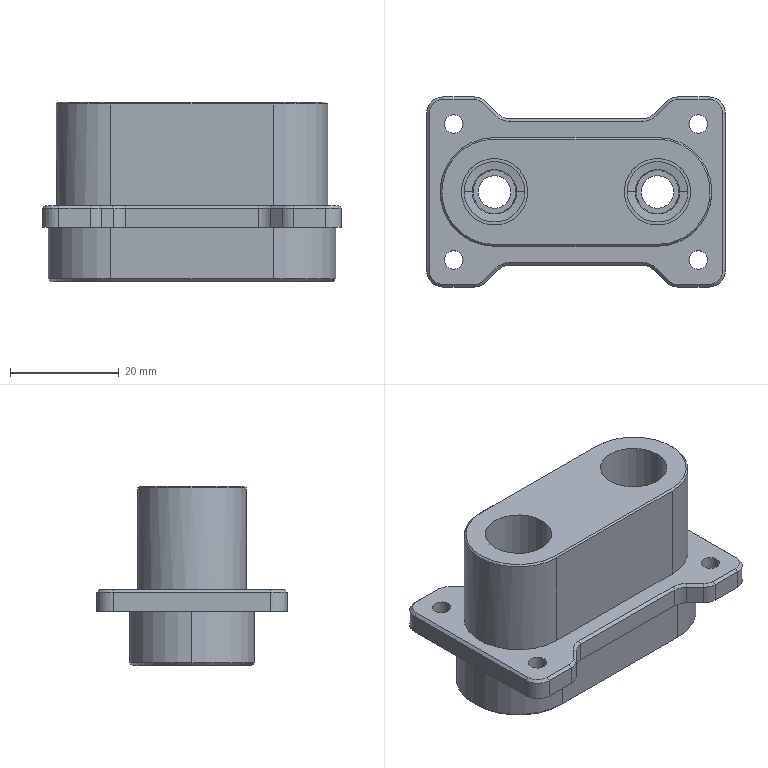NC program | NX | posted with a generic post | part box 55 x 35 x 33 mm
Lines 1800 to 2805 of 2805:
(PLANAR_MILL_3 , TOOL : D50面刀)
N3598 T01 M6
N3600 G54
N3602 G17 G0 G90 X-0.5 Y-54.499 S3500 M3
N3604 G43 Z30. H1
N3606 Z2.
N3608 G94 G1 Z0. F800.
N3610 Y-27.499
N3612 Y27.501
N3614 Y54.501
N3616 Z2.
N3618 G0 Z30.
N3620 M5
(DRILLING_2 , TOOL : D6点钻)
N3622 T03 M6
N3624 G54
N3626 G17 G0 G90 X0. Y15.001 S3000 M3
N3628 G43 Z30. H3
N3630 G94 G81 G98 Z-1.5 F200. R3.
N3632 Y-14.999
N3634 G80
N3636 G0 X0. Y-14.999 Z30.
N3638 M5
(DRILLING_2_COPY , TOOL : D6.5钻头)
N3640 T07 M6
N3642 G54
N3644 G17 G0 G90 X0. Y15.001 S3000 M3
N3646 G43 Z30. H7
N3648 G94 G83 G98 Z-22. F200. Q2. R3.
N3650 Y-14.999
N3652 G80
N3654 G0 X0. Y-14.999 Z30.
N3656 M5
(ADAPTIVE_MILLING_1 , TOOL : D4开粗)
N3658 T09 M6
N3660 G54
N3662 G17 G0 G90 X0. Y15.001 S4500 M3
N3664 G43 Z30. H9
N3666 Z-4.8
N3668 G94 G1 Z-7.8 F600.
N3670 X-0.129 Y14.749
N3672 X-0.242 Y14.488
N3674 G3 X-0.003 Y14.024 R0.405
N3676 X0.939 Y14.457 R0.821
N3678 X-0.266 Y13.936 R-1.092
N3680 X0.641 Y16.006 R1.139
N3682 X-0.135 Y13.792 R-1.2
N3684 X0.189 Y16.285 R-1.257
N3686 X-0.057 Y13.669 R-1.315
N3688 X-0.094 Y16.411 R-1.375
N3690 X0.246 Y13.558 R-1.437
N3692 X-0.727 Y16.35 R-1.502
N3694 X1.283 Y14.005 R-1.573
N3696 X-1.561 Y14.435 R-1.648
N3698 X0.93 Y16.529 R-1.728
N3700 X-0.224 Y13.182 R-1.807
N3702 X-0.149 Y16.926 R-1.885
N3704 X0.765 Y13.148 R-1.963
N3706 X-1.585 Y16.341 R-2.046
N3708 X2.2 Y14.888 R-2.133
N3710 X-1.676 Y13.511 R-2.223
N3712 X1.16 Y17.076 R-2.313
N3714 X-0.504 Y12.623 R-2.402
N3716 X-0.075 Y17.543 R-2.49
N3718 X0.822 Y12.509 R-2.58
N3720 X-1.537 Y17.235 R-2.671
N3722 X2.464 Y13.603 R-2.766
N3724 X-2.879 Y14.768 R-2.865
N3726 X2.637 Y16.518 R-2.965
N3728 X-1.875 Y12.542 R-3.065
N3730 X1.226 Y17.993 R-3.166
N3732 X-0.534 Y11.745 R-3.264
N3734 X0.001 Y18.424 R-3.364
N3736 X0.748 Y11.571 R-3.464
N3738 X-1.722 Y18.179 R-3.566
N3740 X2.827 Y12.556 R-3.671
N3742 X-3.497 Y16.517 R-3.778
N3744 X3.966 Y14.932 R-3.886
N3746 X-3.627 Y13.383 R-3.967
N3748 X-1.737 Y11.432 R4.253
N3750 X0.797 Y11.111 R4.23
N3752 X-0.275 Y18.963 R3.972
N3754 X-2.608 Y17.994 R4.267
N3756 X-3.635 Y16.6 R4.397
N3758 X-3.329 Y16.036 R0.404
N3760 G1 X-2.808 Y15.954
N3762 X-2.66 Y15.93 Z-7.796
N3764 X-2.512 Y15.906 Z-7.785
N3766 X-2.364 Y15.883 Z-7.766
N3768 X-2.216 Y15.859 Z-7.739
N3770 X-2.067 Y15.836 Z-7.705
N3772 X-1.919 Y15.812 Z-7.662
N3774 X-1.771 Y15.789 Z-7.61
N3776 X-1.623 Y15.765 Z-7.55
N3778 X-1.475 Y15.742 Z-7.479
N3780 X-1.327 Y15.718 Z-7.398
N3782 X-1.179 Y15.695 Z-7.305
N3784 X-1.03 Y15.671 Z-7.2
N3786 X-0.882 Y15.647 Z-7.08
N3788 X-0.734 Y15.624 Z-6.942
N3790 X-0.586 Y15.6 Z-6.784
N3792 X-0.438 Y15.577 Z-6.6
N3794 X-0.29 Y15.553 Z-6.38
N3796 X-0.142 Y15.53 Z-6.108
N3798 X0.007 Y15.506 Z-5.737
N3800 X0.155 Y15.483 Z-4.8
N3802 G0 Z30.
N3804 X0. Y-14.999
N3806 Z-4.8
N3808 G1 Z-7.8
N3810 X0.256 Y-15.118
N3812 X0.518 Y-15.221
N3814 G3 X0.976 Y-14.953 R0.405
N3816 X0.369 Y-13.975 R0.857
N3818 X1.084 Y-15.184 R-1.093
N3820 X-1.028 Y-14.397 R1.138
N3822 X1.202 Y-15.154 R-1.199
N3824 X0.162 Y-13.717 R1.254
N3826 X-1.274 Y-14.751 R1.254
N3828 X1.333 Y-14.977 R-1.313
N3830 X-1.405 Y-15.138 R-1.374
N3832 X1.434 Y-14.72 R-1.435
N3834 X-1.388 Y-15.647 R-1.5
N3836 X1.29 Y-14.036 R-1.568
N3838 X-0.646 Y-16.527 R-1.639
N3840 X-1.035 Y-13.545 R-1.718
N3842 X1.721 Y-15.592 R-1.799
N3844 X-1.921 Y-14.837 R-1.878
N3846 X1.97 Y-14.731 R-1.955
N3848 X-1.873 Y-15.89 R-2.035
N3850 X1.394 Y-13.329 R-2.119
N3852 X-0.326 Y-17.203 R-2.207
N3854 X-1.392 Y-13.08 R-2.298
N3856 X2.121 Y-16.152 R-2.39
N3858 X-2.482 Y-14.463 R-2.48
N3860 X2.6 Y-14.786 R-2.57
N3862 X-2.578 Y-15.829 R-2.662
N3864 X2.3 Y-13.389 R-2.754
N3866 X-1.599 Y-17.398 R-2.85
N3868 X0.052 Y-11.975 R-2.949
N3870 X1.394 Y-17.739 R-3.05
N3872 X-2.438 Y-12.886 R-3.152
N3874 X3.002 Y-16.331 R-3.253
N3876 X-3.334 Y-14.244 R-3.354
N3878 X3.496 Y-14.978 R-3.454
N3880 X-3.499 Y-15.895 R-3.557
N3882 X3.177 Y-13.068 R-3.661
N3884 X-2.495 Y-17.874 R-3.766
N3886 X1.602 Y-11.392 R-3.873
N3888 X-2.9 Y-17.696 R3.952
N3890 X1.112 Y-18.811 R4.004
N3892 X2.209 Y-18.299 R5.628
N3894 X3.509 Y-16.854 R4.555
N3896 X3.957 Y-15.368 R4.778
N3898 X-1.887 Y-11.514 R3.976
N3900 X-3.667 Y-13.476 R4.151
N3902 X-3.935 Y-14.461 R4.173
N3904 X-2.9 Y-17.696 R4.009
N3906 X-2.012 Y-18.42 R5.481
N3908 X-0.2 Y-18.967 R4.634
N3910 X0.198 Y-18.501 R0.404
N3912 G1 X0.117 Y-17.979
N3914 X0.094 Y-17.831 Z-7.796
N3916 X0.071 Y-17.683 Z-7.785
N3918 X0.048 Y-17.534 Z-7.766
N3920 X0.025 Y-17.386 Z-7.739
N3922 X0.002 Y-17.238 Z-7.705
N3924 X-0.021 Y-17.09 Z-7.662
N3926 X-0.044 Y-16.942 Z-7.61
N3928 X-0.067 Y-16.793 Z-7.55
N3930 X-0.09 Y-16.645 Z-7.479
N3932 X-0.113 Y-16.497 Z-7.398
N3934 X-0.136 Y-16.349 Z-7.305
N3936 X-0.159 Y-16.2 Z-7.2
N3938 X-0.182 Y-16.052 Z-7.08
N3940 X-0.205 Y-15.904 Z-6.942
N3942 X-0.228 Y-15.756 Z-6.784
N3944 X-0.251 Y-15.607 Z-6.6
N3946 X-0.274 Y-15.459 Z-6.38
N3948 X-0.297 Y-15.311 Z-6.108
N3950 X-0.32 Y-15.163 Z-5.737
N3952 X-0.343 Y-15.015 Z-4.8
N3954 G0 Z30.
N3956 X0.385 Y15.694
N3958 Z-14.808
N3960 G1 X0.366 Y15.659 Z-15.055
N3962 X0.346 Y15.624 Z-15.153
N3964 X0.327 Y15.59 Z-15.225
N3966 X0.308 Y15.555 Z-15.283
N3968 X0.289 Y15.521 Z-15.332
N3970 X0.269 Y15.486 Z-15.374
N3972 X0.25 Y15.451 Z-15.41
N3974 X0.231 Y15.417 Z-15.442
N3976 X0.212 Y15.382 Z-15.469
N3978 X0.192 Y15.347 Z-15.494
N3980 X0.173 Y15.313 Z-15.515
N3982 X0.154 Y15.278 Z-15.534
N3984 X0.135 Y15.244 Z-15.55
N3986 X0.115 Y15.209 Z-15.564
N3988 X0.096 Y15.174 Z-15.575
N3990 X0.077 Y15.14 Z-15.584
N3992 X0.058 Y15.105 Z-15.591
N3994 X0.038 Y15.07 Z-15.596
N3996 X0.019 Y15.036 Z-15.599
N3998 X0. Y15.001 Z-15.6
N4000 X-0.138 Y14.758
N4002 X-0.263 Y14.507
N4004 G3 X-0.003 Y14.009 R0.404
N4006 X1.035 Y14.662 R0.895
N4008 X-0.259 Y13.931 R-1.093
N4010 X0.69 Y15.972 R1.138
N4012 X-0.255 Y13.815 R-1.2
N4014 X0.323 Y16.258 R-1.256
N4016 X-0.104 Y13.671 R-1.314
N4018 X-0.01 Y16.413 R-1.375
N4020 X0.125 Y13.545 R-1.436
N4022 X-0.47 Y16.459 R-1.5
N4024 X0.816 Y13.613 R-1.568
N4026 X-1.524 Y15.656 R-1.64
N4028 X1.466 Y16.021 R-1.718
N4030 X0.776 Y13.371 R-1.792
N4032 X0.564 Y16.712 R1.809
N4034 X-1.709 Y14.424 R1.81
N4036 X-0.985 Y13.495 R1.84
N4038 X-0.425 Y13.703 R0.404
N4040 G1 X-0.213 Y14.227
N4042 X-0.184 Y14.3 Z-15.598
N4044 X-0.154 Y14.374 Z-15.592
N4046 X-0.124 Y14.447 Z-15.582
N4048 X-0.095 Y14.521 Z-15.568
N4050 X-0.065 Y14.594 Z-15.55
N4052 X-0.035 Y14.668 Z-15.527
N4054 X-0.005 Y14.741 Z-15.5
N4056 X0.024 Y14.814 Z-15.468
N4058 X0.054 Y14.888 Z-15.43
N4060 X0.084 Y14.961 Z-15.388
N4062 X0.113 Y15.035 Z-15.339
N4064 X0.143 Y15.108 Z-15.283
N4066 X0.173 Y15.182 Z-15.219
N4068 X0.203 Y15.255 Z-15.147
N4070 X0.232 Y15.329 Z-15.063
N4072 X0.262 Y15.402 Z-14.966
N4074 X0.292 Y15.476 Z-14.85
N4076 X0.321 Y15.549 Z-14.706
N4078 X0.351 Y15.623 Z-14.51
N4080 X0.381 Y15.696 Z-14.015
N4082 G0 Z30.
N4084 X-0.869 Y15.151
N4086 Z-13.743
N4088 G1 X-0.826 Y15.144 Z-14.018
N4090 X-0.783 Y15.136 Z-14.127
N4092 X-0.739 Y15.129 Z-14.207
N4094 X-0.696 Y15.121 Z-14.272
N4096 X-0.652 Y15.114 Z-14.326
N4098 X-0.609 Y15.106 Z-14.373
N4100 X-0.565 Y15.099 Z-14.413
N4102 X-0.522 Y15.091 Z-14.449
N4104 X-0.478 Y15.084 Z-14.48
N4106 X-0.435 Y15.076 Z-14.507
N4108 X-0.391 Y15.069 Z-14.531
N4110 X-0.348 Y15.061 Z-14.551
N4112 X-0.304 Y15.054 Z-14.569
N4114 X-0.261 Y15.046 Z-14.584
N4116 X-0.217 Y15.039 Z-14.597
N4118 X-0.174 Y15.031 Z-14.607
N4120 X-0.13 Y15.024 Z-14.615
N4122 X-0.087 Y15.016 Z-14.621
N4124 X-0.043 Y15.009 Z-14.624
N4126 X0. Y15.001 Z-14.625
N4128 X1.341 Y14.769
N4130 G3 X1.768 Y14.981 R0.405
N4132 X1.68 Y15.869 R1.058
N4134 X-0.699 Y13.247 R-1.887
N4136 X1.87 Y15.278 R1.895
N4138 X1.36 Y16.321 R2.098
N4140 X0.834 Y16.355 R0.441
N4142 G1 X0.203 Y15.881 Z-14.525
N4144 X-0.884 Y15.061 F6000.
N4146 X-1.514 Y14.586 Z-14.625 F600.
N4148 G3 X-1.567 Y13.946 R0.445
N4150 X0.006 Y13.107 R1.979
N4152 G1 X0.614 Y13.212
N4154 G3 X0.935 Y13.651 R0.441
N4156 X0.713 Y14.025 Z-14.568 R0.479
N4158 G1 X0.45 Y14.237 Z-14.525
N4160 X-0.83 Y15.27 F6000.
N4162 X-1.222 Y15.579 Z-14.588 F600.
N4164 G3 X-1.502 Y15.632 Z-14.625 R0.464
N4166 X-1.871 Y15.269 R0.436
N4168 X-1.41 Y14.811 R0.404
N4170 G1 X-0.879 Y14.892
N4172 X-0.792 Y14.906 Z-14.623
N4174 X-0.704 Y14.919 Z-14.616
N4176 X-0.617 Y14.932 Z-14.605
N4178 X-0.53 Y14.946 Z-14.589
N4180 X-0.443 Y14.959 Z-14.569
N4182 X-0.355 Y14.973 Z-14.544
N4184 X-0.268 Y14.986 Z-14.513
N4186 X-0.181 Y14.999 Z-14.478
N4188 X-0.094 Y15.013 Z-14.436
N4190 X-0.007 Y15.026 Z-14.389
N4192 X0.081 Y15.04 Z-14.334
N4194 X0.168 Y15.053 Z-14.272
N4196 X0.255 Y15.066 Z-14.201
N4198 X0.342 Y15.08 Z-14.12
N4200 X0.43 Y15.093 Z-14.027
N4202 X0.517 Y15.107 Z-13.919
N4204 X0.604 Y15.12 Z-13.79
N4206 X0.691 Y15.133 Z-13.629
N4208 X0.779 Y15.147 Z-13.411
N4210 X0.866 Y15.16 Z-12.86
N4212 G0 Z30.
N4214 X-1.778 Y15.285
N4216 Z-10.875
N4218 G1 X-1.689 Y15.271 Z-11.437
N4220 X-1.6 Y15.257 Z-11.659
N4222 X-1.511 Y15.243 Z-11.823
N4224 X-1.422 Y15.228 Z-11.955
N4226 X-1.333 Y15.214 Z-12.065
N4228 X-1.245 Y15.2 Z-12.16
N4230 X-1.156 Y15.186 Z-12.243
N4232 X-1.067 Y15.172 Z-12.315
N4234 X-0.978 Y15.157 Z-12.378
N4236 X-0.889 Y15.143 Z-12.434
N4238 X-0.8 Y15.129 Z-12.482
N4240 X-0.711 Y15.115 Z-12.525
N4242 X-0.622 Y15.101 Z-12.561
N4244 X-0.533 Y15.086 Z-12.592
N4246 X-0.444 Y15.072 Z-12.618
N4248 X-0.356 Y15.058 Z-12.639
N4250 X-0.267 Y15.044 Z-12.655
N4252 X-0.178 Y15.03 Z-12.666
N4254 X-0.089 Y15.015 Z-12.673
N4256 X0. Y15.001 Z-12.675
N4258 X1.43 Y14.773
N4260 G3 X1.866 Y15.015 R0.405
N4262 X1.486 Y16.355 R1.415
N4264 X1.905 Y14.323 R-2.024
N4266 X-0.837 Y17.008 R2.063
N4268 X2.088 Y14.359 R-2.177
N4270 X-1.256 Y16.961 R2.23
N4272 X2.206 Y14.21 R-2.332
N4274 X-1.552 Y16.948 R2.399
N4276 X2.348 Y14.118 R-2.495
N4278 X-1.87 Y16.885 R2.569
N4280 X2.474 Y13.982 R-2.662
N4282 X-1.263 Y17.505 R2.721
N4284 X0.195 Y17.796 R-2.802
N4286 X1.713 Y12.773 R-2.804
N4288 G1 X2.27 Y13.347
N4290 G3 X2.079 Y13.968 R0.404
N4292 G1 X1.576 Y14.144
N4294 X1.434 Y14.194 Z-12.671
N4296 X1.293 Y14.244 Z-12.66
N4298 X1.151 Y14.294 Z-12.641
N4300 X1.01 Y14.344 Z-12.614
N4302 X0.868 Y14.393 Z-12.58
N4304 X0.727 Y14.443 Z-12.537
N4306 X0.585 Y14.493 Z-12.485
N4308 X0.444 Y14.543 Z-12.425
N4310 X0.302 Y14.593 Z-12.354
N4312 X0.161 Y14.642 Z-12.273
N4314 X0.019 Y14.692 Z-12.18
N4316 X-0.122 Y14.742 Z-12.075
N4318 X-0.264 Y14.792 Z-11.955
N4320 X-0.405 Y14.842 Z-11.817
N4322 X-0.547 Y14.891 Z-11.659
N4324 X-0.688 Y14.941 Z-11.475
N4326 X-0.83 Y14.991 Z-11.255
N4328 X-0.971 Y15.041 Z-10.983
N4330 X-1.113 Y15.091 Z-10.612
N4332 X-1.254 Y15.14 Z-9.675
N4334 G0 Z30.
N4336 X2.371 Y15.456
N4338 Z-9.002
N4340 G1 X2.236 Y15.45 Z-9.844
N4342 X2.101 Y15.444 Z-10.178
N4344 X1.966 Y15.437 Z-10.423
N4346 X1.832 Y15.431 Z-10.621
N4348 X1.697 Y15.425 Z-10.787
N4350 X1.562 Y15.419 Z-10.929
N4352 X1.427 Y15.412 Z-11.052
N4354 X1.292 Y15.406 Z-11.16
N4356 X1.158 Y15.4 Z-11.255
N4358 X1.023 Y15.394 Z-11.339
N4360 X0.888 Y15.388 Z-11.411
N4362 X0.753 Y15.381 Z-11.475
N4364 X0.619 Y15.375 Z-11.529
N4366 X0.484 Y15.369 Z-11.576
N4368 X0.349 Y15.363 Z-11.614
N4370 X0.214 Y15.356 Z-11.645
N4372 X0.08 Y15.35 Z-11.669
N4374 X-0.055 Y15.344 Z-11.686
N4376 X-0.19 Y15.338 Z-11.697
N4378 X-0.325 Y15.332 Z-11.7
N4380 X-2.421 Y15.235
N4382 G3 X-2.769 Y15. R0.406
N4384 X-2.632 Y13.669 R1.657
N4386 X1.495 Y17.577 R-2.968
N4388 X-2.973 Y15.349 R3.011
N4390 X-0.449 Y11.883 R2.924
N4392 X-3.058 Y15.817 R-3.154
N4394 X0.563 Y11.714 R3.179
N4396 X-3.144 Y16.152 R-3.339
N4398 X-3.208 Y13.82 R3.199
N4400 X-0.797 Y11.676 R3.526
N4402 X2.393 Y12.559 R3.525
N4404 X3.134 Y16.368 R3.487
N4406 X-0.064 Y18.42 R3.491
N4408 X-3.169 Y16.284 R3.482
N4410 X-3.401 Y14.651 R3.82
N4412 X-2.864 Y14.325 R0.404
N4414 G1 X-2.355 Y14.508
N4416 X-2.214 Y14.558 Z-11.696
N4418 X-2.073 Y14.609 Z-11.685
N4420 X-1.932 Y14.66 Z-11.666
N4422 X-1.791 Y14.71 Z-11.639
N4424 X-1.649 Y14.761 Z-11.605
N4426 X-1.508 Y14.811 Z-11.562
N4428 X-1.367 Y14.862 Z-11.51
N4430 X-1.226 Y14.913 Z-11.45
N4432 X-1.085 Y14.963 Z-11.379
N4434 X-0.943 Y15.014 Z-11.298
N4436 X-0.802 Y15.065 Z-11.205
N4438 X-0.661 Y15.115 Z-11.1
N4440 X-0.52 Y15.166 Z-10.98
N4442 X-0.379 Y15.217 Z-10.842
N4444 X-0.238 Y15.267 Z-10.684
N4446 X-0.096 Y15.318 Z-10.5
N4448 X0.045 Y15.368 Z-10.28
N4450 X0.186 Y15.419 Z-10.008
N4452 X0.327 Y15.47 Z-9.637
N4454 X0.468 Y15.52 Z-8.7
N4456 G0 Z30.
N4458 X-2.288 Y16.542
N4460 Z-6.75
N4462 G1 X-2.228 Y16.405 Z-7.687
N4464 X-2.169 Y16.267 Z-8.058
N4466 X-2.109 Y16.129 Z-8.33
N4468 X-2.05 Y15.992 Z-8.55
N4470 X-1.991 Y15.854 Z-8.734
N4472 X-1.931 Y15.716 Z-8.892
N4474 X-1.872 Y15.578 Z-9.03
N4476 X-1.812 Y15.441 Z-9.15
N4478 X-1.753 Y15.303 Z-9.255
N4480 X-1.693 Y15.165 Z-9.348
N4482 X-1.634 Y15.027 Z-9.429
N4484 X-1.574 Y14.89 Z-9.5
N4486 X-1.515 Y14.752 Z-9.56
N4488 X-1.456 Y14.614 Z-9.612
N4490 X-1.396 Y14.477 Z-9.655
N4492 X-1.337 Y14.339 Z-9.689
N4494 X-1.277 Y14.201 Z-9.716
N4496 X-1.218 Y14.063 Z-9.735
N4498 X-1.158 Y13.926 Z-9.746
N4500 X-1.099 Y13.788 Z-9.75
N4502 X-0.244 Y11.808
N4504 G3 X-0.007 Y11.587 R0.41
N4506 X1.746 Y11.87 R2.296
N4508 X-1.475 Y11.723 R-3.595
N4510 X1.012 Y11.402 R4.173
N4512 X2.401 Y17.934 R3.738
N4514 X-0.902 Y11.303 R-3.794
N4516 X3.34 Y12.865 R3.696
N4518 X2.906 Y12.305 R-3.963
N4520 X3.947 Y14.576 R4.
N4522 X3.863 Y15.929 R3.929
N4524 X-3.627 Y13.383 R-3.971
N4526 X-1.737 Y11.432 R4.253
N4528 G1 X-1.702 Y11.419
N4530 G3 X-1.173 Y11.694 R0.404
N4532 G1 X-1.03 Y12.23
N4534 X-0.991 Y12.375 Z-9.746
N4536 X-0.952 Y12.519 Z-9.735
N4538 X-0.913 Y12.664 Z-9.716
N4540 X-0.875 Y12.809 Z-9.689
N4542 X-0.836 Y12.954 Z-9.655
N4544 X-0.797 Y13.099 Z-9.612
N4546 X-0.758 Y13.244 Z-9.56
N4548 X-0.719 Y13.389 Z-9.5
N4550 X-0.681 Y13.534 Z-9.429
N4552 X-0.642 Y13.679 Z-9.348
N4554 X-0.603 Y13.824 Z-9.255
N4556 X-0.564 Y13.968 Z-9.15
N4558 X-0.525 Y14.113 Z-9.03
N4560 X-0.487 Y14.258 Z-8.892
N4562 X-0.448 Y14.403 Z-8.734
N4564 X-0.409 Y14.548 Z-8.55
N4566 X-0.37 Y14.693 Z-8.33
N4568 X-0.331 Y14.838 Z-8.058
N4570 X-0.293 Y14.983 Z-7.687
N4572 X-0.254 Y15.128 Z-6.75
N4574 G0 Z30.
N4576 X-0.707 Y-14.623
N4578 Z-14.799
N4580 G1 X-0.672 Y-14.641 Z-15.049
N4582 X-0.637 Y-14.66 Z-15.148
N4584 X-0.601 Y-14.679 Z-15.221
N4586 X-0.566 Y-14.698 Z-15.28
N4588 X-0.53 Y-14.717 Z-15.329
N4590 X-0.495 Y-14.736 Z-15.371
N4592 X-0.46 Y-14.754 Z-15.408
N4594 X-0.424 Y-14.773 Z-15.44
N4596 X-0.389 Y-14.792 Z-15.468
N4598 X-0.354 Y-14.811 Z-15.493
N4600 X-0.318 Y-14.83 Z-15.514
N4602 X-0.283 Y-14.848 Z-15.533
N4604 X-0.248 Y-14.867 Z-15.549
N4606 X-0.212 Y-14.886 Z-15.563
N4608 X-0.177 Y-14.905 Z-15.575
N4610 X-0.141 Y-14.924 Z-15.584
N4612 X-0.106 Y-14.942 Z-15.591
N4614 X-0.071 Y-14.961 Z-15.596
N4616 X-0.035 Y-14.98 Z-15.599
N4618 X0. Y-14.999 Z-15.6
N4620 X0.246 Y-15.133
N4622 X0.5 Y-15.254
N4624 G3 X0.989 Y-15.001 R0.404
N4626 X0.969 Y-14.558 R0.61
N4628 X-0.684 Y-14.148 R1.058
N4630 X1.037 Y-15.351 R-1.093
N4632 X-0.032 Y-13.81 R1.113
N4634 X1.028 Y-15.609 R-1.192
N4636 X-0.369 Y-13.757 R1.234
N4638 X0.991 Y-15.844 R-1.298
N4640 X-0.537 Y-13.698 R1.35
N4642 X0.987 Y-16.015 R-1.412
N4644 X-0.639 Y-13.612 R1.468
N4646 X0.952 Y-16.205 R-1.531
N4648 X-0.598 Y-13.46 R1.592
N4650 X0.848 Y-16.429 R-1.657
N4652 X-0.562 Y-13.309 R1.721
N4654 X0.661 Y-16.667 R-1.788
N4656 X1.295 Y-16.249 R2.062
N4658 X1.558 Y-14.082 R1.848
N4660 X-0.535 Y-13.271 R1.868
N4662 X-1.694 Y-14.366 R1.939
N4664 X-1.587 Y-15.83 R1.783
N4666 X-1.31 Y-16.22 R0.989
N4668 G1 X-1.249 Y-16.282
N4670 G3 X-0.889 Y-16.554 R0.935
N4672 G1 X-0.769 Y-16.617
N4674 G3 X-0.314 Y-16.761 R0.988
N4676 X1.522 Y-15.95 R1.752
N4678 G1 X1.616 Y-15.802
N4680 G3 X1.349 Y-15.255 R0.404
N4682 G1 X0.797 Y-15.107
N4684 X0.72 Y-15.086 Z-15.598
N4686 X0.643 Y-15.065 Z-15.592
N4688 X0.566 Y-15.044 Z-15.582
N4690 X0.489 Y-15.023 Z-15.568
N4692 X0.412 Y-15.002 Z-15.549
N4694 X0.335 Y-14.982 Z-15.526
N4696 X0.258 Y-14.961 Z-15.499
N4698 X0.18 Y-14.94 Z-15.467
N4700 X0.103 Y-14.919 Z-15.429
N4702 X0.026 Y-14.898 Z-15.386
N4704 X-0.051 Y-14.877 Z-15.337
N4706 X-0.128 Y-14.857 Z-15.281
N4708 X-0.205 Y-14.836 Z-15.217
N4710 X-0.282 Y-14.815 Z-15.143
N4712 X-0.359 Y-14.794 Z-15.059
N4714 X-0.436 Y-14.773 Z-14.961
N4716 X-0.514 Y-14.753 Z-14.844
N4718 X-0.591 Y-14.732 Z-14.699
N4720 X-0.668 Y-14.711 Z-14.501
N4722 X-0.745 Y-14.69 Z-14.003
N4724 G0 Z30.
N4726 X-0.862 Y-14.82
N4728 Z-13.745
N4730 G1 X-0.819 Y-14.829 Z-14.02
N4732 X-0.775 Y-14.838 Z-14.129
N4734 X-0.732 Y-14.847 Z-14.209
N4736 X-0.689 Y-14.856 Z-14.273
N4738 X-0.646 Y-14.865 Z-14.327
N4740 X-0.603 Y-14.874 Z-14.373
N4742 X-0.56 Y-14.883 Z-14.414
N4744 X-0.517 Y-14.892 Z-14.449
N4746 X-0.474 Y-14.901 Z-14.48
N4748 X-0.431 Y-14.91 Z-14.507
N4750 X-0.388 Y-14.918 Z-14.531
N4752 X-0.345 Y-14.927 Z-14.552
N4754 X-0.302 Y-14.936 Z-14.569
N4756 X-0.258 Y-14.945 Z-14.584
N4758 X-0.215 Y-14.954 Z-14.597
N4760 X-0.172 Y-14.963 Z-14.607
N4762 X-0.129 Y-14.972 Z-14.615
N4764 X-0.086 Y-14.981 Z-14.621
N4766 X-0.043 Y-14.99 Z-14.624
N4768 X0. Y-14.999 Z-14.625
N4770 X1.33 Y-15.274
N4772 G3 X1.79 Y-15.02 R0.405
N4774 X1.668 Y-14.109 R1.205
N4776 X-1.122 Y-16.519 R-1.888
N4778 X1.867 Y-14.703 R1.896
N4780 G1 X1.825 Y-14.559
N4782 G3 X1.503 Y-14.277 R0.402
N4784 X1.148 Y-14.39 Z-14.576 R0.448
N4786 G1 X0.818 Y-14.625 Z-14.525
N4788 X0.311 Y-14.981 F6000.
N4790 X0.212 Y-15.011
N4792 X0.109 Y-15.019
N4794 X-0.054 Y-15.006
N4796 X-0.217 Y-15.007
N4798 X-0.861 Y-15.195
N4800 X-1.455 Y-15.376 Z-14.604 F600.
N4802 X-1.525 Y-15.421 Z-14.614
N4804 X-1.589 Y-15.475 Z-14.625
N4806 G3 X-1.659 Y-15.89 R0.402
N4808 X0.332 Y-16.844 R1.847
N4810 X1.409 Y-16.235 R1.717
N4812 G1 X1.601 Y-16.008
N4814 G3 X1.368 Y-15.382 R0.404
N4816 G1 X0.848 Y-15.254
N4818 X0.762 Y-15.232 Z-14.623
N4820 X0.677 Y-15.211 Z-14.616
N4822 X0.591 Y-15.19 Z-14.605
N4824 X0.505 Y-15.169 Z-14.589
N4826 X0.42 Y-15.148 Z-14.569
N4828 X0.334 Y-15.126 Z-14.544
N4830 X0.249 Y-15.105 Z-14.513
N4832 X0.163 Y-15.084 Z-14.478
N4834 X0.077 Y-15.063 Z-14.436
N4836 X-0.008 Y-15.042 Z-14.389
N4838 X-0.094 Y-15.021 Z-14.334
N4840 X-0.179 Y-14.999 Z-14.272
N4842 X-0.265 Y-14.978 Z-14.202
N4844 X-0.351 Y-14.957 Z-14.121
N4846 X-0.436 Y-14.936 Z-14.028
N4848 X-0.522 Y-14.915 Z-13.92
N4850 X-0.607 Y-14.893 Z-13.79
N4852 X-0.693 Y-14.872 Z-13.63
N4854 X-0.779 Y-14.851 Z-13.412
N4856 X-0.864 Y-14.83 Z-12.861
N4858 G0 Z30.
N4860 X-0.27 Y-16.774
N4862 Z-10.88
N4864 G1 X-0.256 Y-16.685 Z-11.44
N4866 X-0.243 Y-16.596 Z-11.662
N4868 X-0.229 Y-16.508 Z-11.825
N4870 X-0.216 Y-16.419 Z-11.957
N4872 X-0.202 Y-16.33 Z-12.067
N4874 X-0.189 Y-16.241 Z-12.162
N4876 X-0.175 Y-16.153 Z-12.244
N4878 X-0.162 Y-16.064 Z-12.316
N4880 X-0.148 Y-15.975 Z-12.379
N4882 X-0.135 Y-15.886 Z-12.434
N4884 X-0.121 Y-15.798 Z-12.483
N4886 X-0.108 Y-15.709 Z-12.525
N4888 X-0.094 Y-15.62 Z-12.561
N4890 X-0.081 Y-15.531 Z-12.592
N4892 X-0.067 Y-15.443 Z-12.618
N4894 X-0.054 Y-15.354 Z-12.639
N4896 X-0.04 Y-15.265 Z-12.655
N4898 X-0.027 Y-15.176 Z-12.666
N4900 X-0.013 Y-15.088 Z-12.673
N4902 X0. Y-14.999 Z-12.675
N4904 X0.217 Y-13.568
N4906 G3 X-0.013 Y-13.141 R0.405
N4908 X-1.218 Y-13.398 R1.301
N4910 X0.937 Y-13.202 R-2.024
N4912 X-1.342 Y-13.316 R2.146
N4914 X2.011 Y-14.172 R-2.17
N4916 X-1.686 Y-13.424 R2.281
N4918 X1.713 Y-13.421 R-2.325
N4920 X-1.811 Y-16.706 R-2.409
N4922 X0.815 Y-12.621 R-2.497
N4924 X-1.873 Y-16.879 R2.571
N4926 X0.993 Y-12.51 R-2.663
N4928 X-2.552 Y-16.146 R2.716
N4930 X1.15 Y-17.551 R2.8
N4932 X-2.552 Y-16.146 R-2.8
N4934 X1.625 Y-12.713 R-2.802
N4936 G1 X1.555 Y-12.659
N4938 G3 X0.951 Y-12.873 R0.404
N4940 G1 X0.785 Y-13.385
N4942 X0.738 Y-13.528 Z-12.671
N4944 X0.692 Y-13.67 Z-12.66
N4946 X0.646 Y-13.813 Z-12.641
N4948 X0.599 Y-13.956 Z-12.614
N4950 X0.553 Y-14.098 Z-12.58
N4952 X0.507 Y-14.241 Z-12.537
N4954 X0.46 Y-14.384 Z-12.485
N4956 X0.414 Y-14.526 Z-12.425
N4958 X0.368 Y-14.669 Z-12.354
N4960 X0.321 Y-14.812 Z-12.273
N4962 X0.275 Y-14.954 Z-12.18
N4964 X0.229 Y-15.097 Z-12.075
N4966 X0.182 Y-15.24 Z-11.955
N4968 X0.136 Y-15.382 Z-11.817
N4970 X0.09 Y-15.525 Z-11.659
N4972 X0.043 Y-15.668 Z-11.475
N4974 X-0.003 Y-15.81 Z-11.255
N4976 X-0.049 Y-15.953 Z-10.983
N4978 X-0.096 Y-16.096 Z-10.612
N4980 X-0.142 Y-16.238 Z-9.675
N4982 G0 Z30.
N4984 X2.41 Y-14.982
N4986 Z-8.954
N4988 G1 X2.273 Y-14.983 Z-9.811
N4990 X2.135 Z-10.151
N4992 X1.998 Y-14.984 Z-10.4
N4994 X1.861 Y-14.985 Z-10.601
N4996 X1.723 Y-14.986 Z-10.77
N4998 X1.586 Y-14.987 Z-10.915
N5000 X1.449 Y-14.988 Z-11.041
N5002 X1.311 Y-14.989 Z-11.151
N5004 X1.174 Y-14.99 Z-11.247
N5006 X1.037 Z-11.332
N5008 X0.9 Y-14.991 Z-11.406
N5010 X0.762 Y-14.992 Z-11.471
N5012 X0.625 Y-14.993 Z-11.526
N5014 X0.488 Y-14.994 Z-11.574
N5016 X0.35 Y-14.995 Z-11.613
N5018 X0.213 Y-14.996 Z-11.645
N5020 X0.076 Y-14.997 Z-11.669
N5022 X-0.062 Z-11.686
N5024 X-0.199 Y-14.998 Z-11.697
N5026 X-0.336 Y-14.999 Z-11.7
N5028 X-2.389 Y-15.012
N5030 G3 X-2.781 Y-15.33 R0.405
N5032 X-2.234 Y-16.943 R2.018
N5034 X-2.94 Y-14.56 R-2.973
N5036 X0.114 Y-18.147 R2.948
N5038 X-3.124 Y-14.486 R-3.154
N5040 X0.833 Y-18.227 R3.177
N5042 X-3.254 Y-14.201 R-3.338
N5044 X-3.208 Y-16.18 R3.137
N5046 X-0.797 Y-18.324 R3.526
N5048 X2.425 Y-17.408 R3.52
N5050 X3.418 Y-15.068 R3.616
N5052 X2.521 Y-12.69 R3.616
N5054 X0.617 Y-11.634 R3.679
N5056 X-3.375 Y-15.474 R3.425
N5058 X-2.955 Y-15.791 R0.405
N5060 G1 X-2.303 Y-15.749
N5062 X-2.154 Y-15.74 Z-11.696
N5064 X-2.004 Y-15.73 Z-11.685
N5066 X-1.854 Y-15.721 Z-11.666
N5068 X-1.705 Y-15.711 Z-11.639
N5070 X-1.555 Y-15.702 Z-11.605
N5072 X-1.405 Y-15.692 Z-11.562
N5074 X-1.255 Y-15.682 Z-11.51
N5076 X-1.106 Y-15.673 Z-11.45
N5078 X-0.956 Y-15.663 Z-11.379
N5080 X-0.806 Y-15.654 Z-11.298
N5082 X-0.657 Y-15.644 Z-11.205
N5084 X-0.507 Y-15.634 Z-11.1
N5086 X-0.357 Y-15.625 Z-10.98
N5088 X-0.208 Y-15.615 Z-10.842
N5090 X-0.058 Y-15.606 Z-10.684
N5092 X0.092 Y-15.596 Z-10.5
N5094 X0.241 Y-15.587 Z-10.28
N5096 X0.391 Y-15.577 Z-10.008
N5098 X0.541 Y-15.567 Z-9.637
N5100 X0.691 Y-15.558 Z-8.7
N5102 G0 Z30.
N5104 X-2.069 Y-13.396
N5106 Z-6.75
N5108 G1 X-2.017 Y-13.536 Z-7.687
N5110 X-1.965 Y-13.677 Z-8.058
N5112 X-1.913 Y-13.818 Z-8.33
N5114 X-1.861 Y-13.958 Z-8.55
N5116 X-1.809 Y-14.099 Z-8.734
N5118 X-1.757 Y-14.24 Z-8.892
N5120 X-1.705 Y-14.38 Z-9.03
N5122 X-1.653 Y-14.521 Z-9.15
N5124 X-1.601 Y-14.662 Z-9.255
N5126 X-1.549 Y-14.802 Z-9.348
N5128 X-1.496 Y-14.943 Z-9.429
N5130 X-1.444 Y-15.084 Z-9.5
N5132 X-1.392 Y-15.224 Z-9.56
N5134 X-1.34 Y-15.365 Z-9.612
N5136 X-1.288 Y-15.506 Z-9.655
N5138 X-1.236 Y-15.646 Z-9.689
N5140 X-1.184 Y-15.787 Z-9.716
N5142 X-1.132 Y-15.928 Z-9.735
N5144 X-1.08 Y-16.068 Z-9.746
N5146 X-1.028 Y-16.209 Z-9.75
N5148 X-0.312 Y-18.145
N5150 G3 X0.066 Y-18.409 R0.405
N5152 X2.195 Y-17.835 R2.605
N5154 X-0.666 Y-18.534 R-3.595
N5156 X3.626 Y-16.089 R3.498
N5158 X-0.834 Y-18.708 R-3.788
N5160 X3.412 Y-17.003 R3.692
N5162 X-3.579 Y-13.304 R-3.959
N5164 X-2.1 Y-18.356 R3.96
N5166 X3.776 Y-16.178 R3.955
N5168 X3.756 Y-13.743 R3.735
N5170 X-2.923 Y-17.666 R-3.959
N5172 X-1.194 Y-18.784 R4.225
N5174 X-0.67 Y-18.42 R0.404
N5176 G1 X-0.641 Y-17.882
N5178 X-0.633 Y-17.733 Z-9.746
N5180 X-0.625 Y-17.583 Z-9.735
N5182 X-0.617 Y-17.433 Z-9.716
N5184 X-0.609 Y-17.283 Z-9.689
N5186 X-0.601 Y-17.134 Z-9.655
N5188 X-0.593 Y-16.984 Z-9.612
N5190 X-0.585 Y-16.834 Z-9.56
N5192 X-0.577 Y-16.684 Z-9.5
N5194 X-0.569 Y-16.534 Z-9.429
N5196 X-0.561 Y-16.385 Z-9.348
N5198 X-0.553 Y-16.235 Z-9.255
N5200 X-0.545 Y-16.085 Z-9.15
N5202 X-0.536 Y-15.935 Z-9.03
N5204 X-0.528 Y-15.785 Z-8.892
N5206 X-0.52 Y-15.636 Z-8.734
N5208 X-0.512 Y-15.486 Z-8.55
N5210 X-0.504 Y-15.336 Z-8.33
N5212 X-0.496 Y-15.186 Z-8.058
N5214 X-0.488 Y-15.037 Z-7.687
N5216 X-0.48 Y-14.887 Z-6.75
N5218 G0 Z30.
N5220 M5
(DRILLING_2_COPY_COPY , TOOL : D7.9成型刀)
N5222 T10 M6
N5224 G54
N5226 G17 G0 G90 X0. Y15.001 S4000 M3
N5228 G43 Z30. H10
N5230 G94 G81 G98 Z-15.75 F80. R3.
N5232 Y-14.999
N5234 G80
N5236 G0 X0. Y-14.999 Z30.
N5238 M5
(PLANAR_MILL_5 , TOOL : D6点钻)
N5240 T03 M6
N5242 G54
N5244 G17 G0 G90 X-13.2 Y13.001 S3500 M3
N5246 G43 Z30. H3
N5248 Z0.5
N5250 G94 G1 Z-1.5 F800.
N5252 G3 X-11.2 Y15.001 R2.
N5254 G2 X0. Y26.201 R11.2
N5256 X11.2 Y15.001 R11.2
N5258 G1 Y-14.999
N5260 G2 X0. Y-26.199 R11.2
N5262 X-11.2 Y-14.999 R11.2
N5264 G1 Y15.001
N5266 G3 X-13.2 Y17.001 R2.
N5268 G1 Z0.5
N5270 G0 Z30.
(PLANAR_MILL_5_COPY , TOOL : D6点钻)
N5272 X-21. Y16.744
N5274 Z-19.
N5276 G1 Z-21.
N5278 G3 X-19. Y18.744 R2.
N5280 G1 Y24.501
N5282 G2 X-14.5 Y29.001 R4.5
N5284 G1 X14.5
N5286 G2 X19. Y24.501 R4.5
N5288 G1 Y18.744
N5290 G2 X17.682 Y15.562 R4.5
N5292 G1 X15.439 Y13.319
N5294 G3 X15. Y12.259 R1.5
N5296 G1 Y-12.256
N5298 G3 X15.439 Y-13.317 R1.5
N5300 G1 X17.682 Y-15.559
N5302 G2 X19. Y-18.741 R4.5
N5304 G1 Y-24.499
N5306 G2 X14.5 Y-28.999 R4.5
N5308 G1 X-14.5
N5310 G2 X-19. Y-24.499 R4.5
N5312 G1 Y-18.741
N5314 G2 X-17.682 Y-15.559 R4.5
N5316 G1 X-15.439 Y-13.317
N5318 G3 X-15. Y-12.256 R1.5
N5320 G1 Y12.259
N5322 G3 X-15.439 Y13.319 R1.5
N5324 G1 X-17.682 Y15.562
N5326 G2 X-19. Y18.744 R4.5
N5328 G3 X-21. Y20.744 R2.
N5330 G1 Z-19.
N5332 G0 Z30.
(DRILLING_3 , TOOL : D6点钻)
N5334 X-12.5 Y22.501 S3000
N5336 G81 G98 Z-20.7 F200. R-16.
N5338 Y-22.499
N5340 X12.5
N5342 Y22.501
N5344 G80
N5346 G0 X12.5 Y22.501 Z30.
N5348 M5
(PLANAR_MILL_7 , TOOL : D6精光)
N5350 T06 M6
N5352 G54
N5354 G17 G0 G90 X-19.2 Y13.001 S5500 M3
N5356 G43 Z30. H6
N5358 Z-17.
N5360 G94 G1 Z-19. F800.
N5362 G3 X-17.2 Y15.001 R2.
N5364 G2 X0. Y32.201 R17.2
N5366 X17.2 Y15.001 R17.2
N5368 G1 Y-14.999
N5370 G2 X0. Y-32.199 R17.2
N5372 X-17.2 Y-14.999 R17.2
N5374 G1 Y15.001
N5376 G3 X-19.2 Y17.001 R2.
N5378 G1 X-15. Y13.001
N5380 G3 X-13. Y15.001 R2.
N5382 G2 X0. Y28.001 R13.
N5384 X13. Y15.001 R13.
N5386 G1 Y-14.999
N5388 G2 X0. Y-27.999 R13.
N5390 X-13. Y-14.999 R13.
N5392 G1 Y15.001
N5394 G3 X-15. Y17.001 R2.
N5396 G1 X-19.032 Y17.539
N5398 Z-17.
N5400 G0 Z30.
(PLANAR_MILL_7_COPY , TOOL : D6精光)
N5402 X-17.197 Y13.036
N5404 Z-17.
N5406 G1 Z-19.
N5408 G41 X-17. Y13.001 D6
N5410 X-15.
N5412 G3 X-13. Y15.001 R2.
N5414 G2 X0. Y28.001 R13.
N5416 X13. Y15.001 R13.
N5418 G1 Y-14.999
N5420 G2 X0. Y-27.999 R13.
N5422 X-13. Y-14.999 R13.
N5424 G1 Y15.001
N5426 G3 X-15. Y17.001 R2.
N5428 G1 X-16.882
N5430 G40
N5432 X-17.079 Y16.967
N5434 Z-17.
N5436 G0 Z30.
N5438 M5
(PLANAR_MILL_4 , TOOL : D4精光)
N5440 T11 M6
N5442 G54
N5444 G17 G0 G90 X2. Y15.719 S5500 M3
N5446 G43 Z30. H11
N5448 Z-7.9
N5450 G94 G1 Z-9.9 F200.
N5452 Y17.126
N5454 G3 X0. Y19.126 R2.
N5456 X-4.125 Y15.001 R4.125
N5458 X0. Y19.126 R-4.125
N5460 X-2. Y17.126 R2.
N5462 G1 Y15.719
N5464 Z-7.9
N5466 G0 Z30.
N5468 Y-15.717
N5470 Z-7.9
N5472 G1 Z-9.9
N5474 Y-17.124
N5476 G3 X0. Y-19.124 R2.
N5478 X4.125 Y-14.999 R4.125
N5480 X0. Y-19.124 R-4.125
N5482 X2. Y-17.124 R2.
N5484 G1 Y-15.717
N5486 Z-7.9
N5488 G0 Z30.
(PLANAR_MILL_4_COPY , TOOL : D4精光)
N5490 X1.237 Y-14.024
N5492 Z-10.7
N5494 G1 Z-12.7
N5496 X2. Y-13.424
N5498 G3 X0. Y-11.424 R2.
N5500 X-3.575 Y-14.999 R3.575
N5502 X0. Y-11.424 R-3.575
N5504 X-2. Y-13.424 R2.
N5506 G1 X-1.237 Y-14.024
N5508 Z-10.7
N5510 G0 Z30.
N5512 Y14.027
N5514 Z-10.7
N5516 G1 Z-12.7
N5518 X-2. Y13.426
N5520 G3 X0. Y11.426 R2.
N5522 X3.575 Y15.001 R3.575
N5524 X0. Y11.426 R-3.575
N5526 X2. Y13.426 R2.
N5528 G1 X1.237 Y14.027
N5530 Z-10.7
N5532 G0 Z30.
N5534 M5
N5536 M2